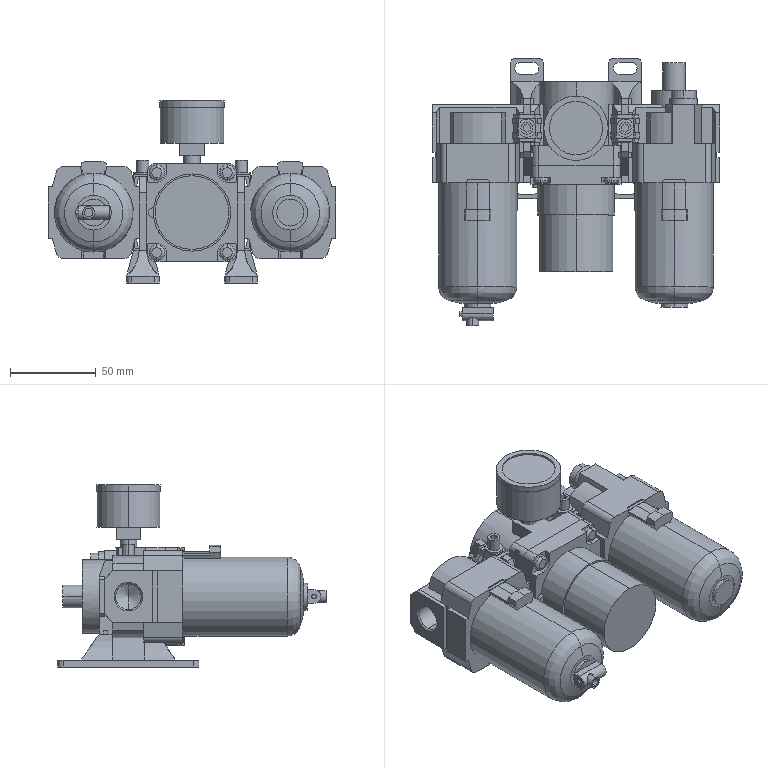Part | SolidWorks | 14 solids | 872 faces | box 167.4 x 156.1 x 106 mm | volume 703605 mm3 | plane 606 | cylinder 186 | cone 68 | torus 12 | commonest cylinder face diameters 7 x18 4 x17 8 x17 3.242 x16 14.95 x12 46 x10